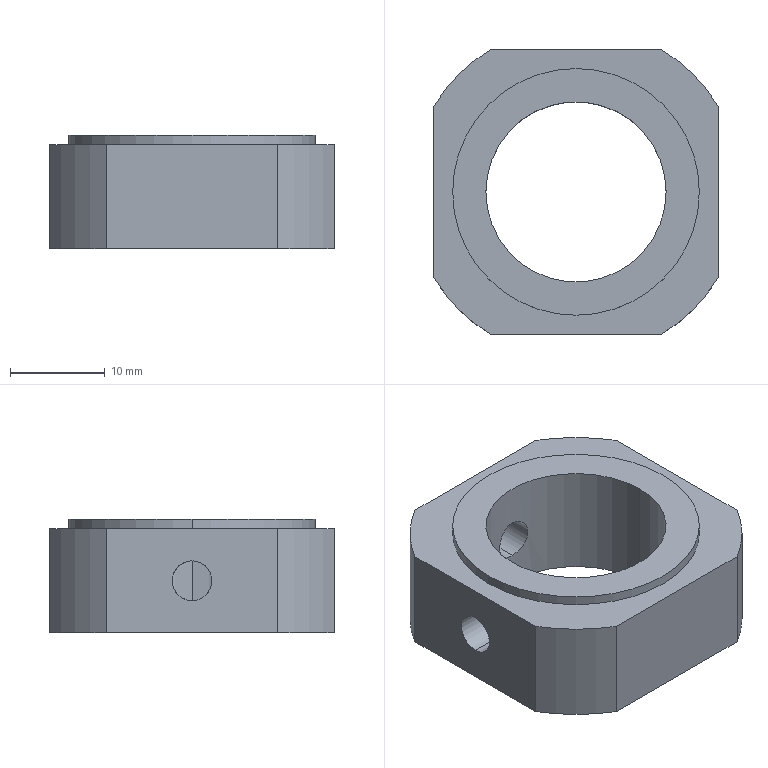Part | SolidWorks | features HoleWzd 2, ICE 2, Extrusion 1 | 1 solid | 19 faces | box 30 x 30 x 12 mm | volume 6216 mm3 | cylinder 12 | plane 7 | commonest cylinder face diameters 4.2 x4 35 x4 19 x2 26 x2
STEP:
#1=CARTESIAN_POINT('',(0.,9.5,3.4));
#2=VERTEX_POINT('',#1);
#3=CARTESIAN_POINT('',(0.,9.5,7.6));
#4=VERTEX_POINT('',#3);
#5=CARTESIAN_POINT('',(0.,9.5,3.4));
#6=CARTESIAN_POINT('',(-0.2745,9.5,3.4));
#7=CARTESIAN_POINT('',(-0.5516,9.487,3.455));
#8=CARTESIAN_POINT('',(-0.9309,9.455,3.613));
#9=CARTESIAN_POINT('',(-1.054,9.442,3.678));
#10=CARTESIAN_POINT('',(-1.282,9.414,3.831));
#11=CARTESIAN_POINT('',(-1.387,9.399,3.918));
#12=CARTESIAN_POINT('',(-1.581,9.368,4.111));
#13=CARTESIAN_POINT('',(-1.669,9.352,4.219));
#14=CARTESIAN_POINT('',(-1.821,9.324,4.446));
#15=CARTESIAN_POINT('',(-1.886,9.311,4.566));
#16=CARTESIAN_POINT('',(-2.045,9.278,4.949));
#17=CARTESIAN_POINT('',(-2.1,9.265,5.222));
#18=CARTESIAN_POINT('',(-2.1,9.265,5.638));
#19=CARTESIAN_POINT('',(-2.087,9.268,5.774));
#20=CARTESIAN_POINT('',(-2.033,9.28,6.044));
#21=CARTESIAN_POINT('',(-1.992,9.289,6.178));
#22=CARTESIAN_POINT('',(-1.887,9.311,6.431));
#23=CARTESIAN_POINT('',(-1.823,9.324,6.552));
#24=CARTESIAN_POINT('',(-1.67,9.352,6.78));
#25=CARTESIAN_POINT('',(-1.582,9.368,6.888));
#26=CARTESIAN_POINT('',(-1.293,9.414,7.177));
#27=CARTESIAN_POINT('',(-1.06,9.444,7.334));
#28=CARTESIAN_POINT('',(-0.6808,9.476,7.491));
#29=CARTESIAN_POINT('',(-0.5473,9.485,7.532));
#30=CARTESIAN_POINT('',(-0.2765,9.497,7.586));
#31=CARTESIAN_POINT('',(-0.1392,9.5,7.6));
#32=CARTESIAN_POINT('',(0.,9.5,7.6));
#33=B_SPLINE_CURVE_WITH_KNOTS('',3,(#5,#6,#7,#8,#9,#10,#11,#12,#13,#14,#15,#16,#17,#18,#19,#20,#21,#22,#23,#24,#25,#26,#27,#28,#29,#30,#31,#32),.UNSPECIFIED.,.F.,.F.,(4,2,2,2,2,2,2,2,2,2,2,2,2,4),(0.006586,0.007409,0.00782,0.008232,0.008644,0.009055,0.009878,0.01029,0.0107,0.01111,0.01152,0.01235,0.01276,0.01317),.UNSPECIFIED.);
#34=EDGE_CURVE('',#2,#4,#33,.T.);
#35=ORIENTED_EDGE('',*,*,#34,.F.);
#36=CARTESIAN_POINT('',(0.,15.,3.4));
#37=VERTEX_POINT('',#36);
#38=CARTESIAN_POINT('',(0.,15.,3.4));
#39=DIRECTION('',(0.,1.,0.));
#40=VECTOR('',#39,1000.);
#41=LINE('',#38,#40);
#42=EDGE_CURVE('',#2,#37,#41,.T.);
#43=ORIENTED_EDGE('',*,*,#42,.T.);
#44=CARTESIAN_POINT('',(0.,15.,7.6));
#45=VERTEX_POINT('',#44);
#46=CARTESIAN_POINT('',(0.,15.,5.5));
#47=DIRECTION('',(0.,1.,0.));
#48=DIRECTION('',(0.,0.,1.));
#49=AXIS2_PLACEMENT_3D('',#46,#47,#48);
#50=CIRCLE('',#49,2.1);
#51=EDGE_CURVE('',#37,#45,#50,.T.);
#52=ORIENTED_EDGE('',*,*,#51,.T.);
#53=CARTESIAN_POINT('',(0.,15.,7.6));
#54=DIRECTION('',(0.,1.,0.));
#55=VECTOR('',#54,1000.);
#56=LINE('',#53,#55);
#57=EDGE_CURVE('',#4,#45,#56,.T.);
#58=ORIENTED_EDGE('',*,*,#57,.F.);
#59=EDGE_LOOP('',(#35,#43,#52,#58));
#60=FACE_OUTER_BOUND('',#59,.T.);
#61=CARTESIAN_POINT('',(0.,15.,5.5));
#62=DIRECTION('',(0.,1.,0.));
#63=DIRECTION('',(0.,0.,1.));
#64=AXIS2_PLACEMENT_3D('',#61,#62,#63);
#65=CYLINDRICAL_SURFACE('',#64,2.1);
#66=ADVANCED_FACE('',(#60),#65,.F.);
#67=CARTESIAN_POINT('',(-9.5,0.,3.4));
#68=VERTEX_POINT('',#67);
#69=CARTESIAN_POINT('',(-9.5,0.,7.6));
#70=VERTEX_POINT('',#69);
#71=CARTESIAN_POINT('',(-9.5,0.,3.4));
#72=CARTESIAN_POINT('',(-9.5,-0.2745,3.4));
#73=CARTESIAN_POINT('',(-9.487,-0.5516,3.455));
#74=CARTESIAN_POINT('',(-9.455,-0.9309,3.613));
#75=CARTESIAN_POINT('',(-9.442,-1.054,3.678));
#76=CARTESIAN_POINT('',(-9.414,-1.282,3.831));
#77=CARTESIAN_POINT('',(-9.399,-1.387,3.918));
#78=CARTESIAN_POINT('',(-9.368,-1.581,4.111));
#79=CARTESIAN_POINT('',(-9.352,-1.669,4.219));
#80=CARTESIAN_POINT('',(-9.324,-1.821,4.446));
#81=CARTESIAN_POINT('',(-9.311,-1.886,4.566));
#82=CARTESIAN_POINT('',(-9.278,-2.045,4.949));
#83=CARTESIAN_POINT('',(-9.265,-2.1,5.222));
#84=CARTESIAN_POINT('',(-9.265,-2.1,5.638));
#85=CARTESIAN_POINT('',(-9.268,-2.087,5.774));
#86=CARTESIAN_POINT('',(-9.28,-2.033,6.044));
#87=CARTESIAN_POINT('',(-9.289,-1.992,6.178));
#88=CARTESIAN_POINT('',(-9.311,-1.887,6.431));
#89=CARTESIAN_POINT('',(-9.324,-1.823,6.552));
#90=CARTESIAN_POINT('',(-9.352,-1.67,6.78));
#91=CARTESIAN_POINT('',(-9.368,-1.582,6.888));
#92=CARTESIAN_POINT('',(-9.414,-1.293,7.177));
#93=CARTESIAN_POINT('',(-9.444,-1.06,7.334));
#94=CARTESIAN_POINT('',(-9.476,-0.6808,7.491));
#95=CARTESIAN_POINT('',(-9.485,-0.5473,7.532));
#96=CARTESIAN_POINT('',(-9.497,-0.2765,7.586));
#97=CARTESIAN_POINT('',(-9.5,-0.1392,7.6));
#98=CARTESIAN_POINT('',(-9.5,0.,7.6));
#99=B_SPLINE_CURVE_WITH_KNOTS('',3,(#71,#72,#73,#74,#75,#76,#77,#78,#79,#80,#81,#82,#83,#84,#85,#86,#87,#88,#89,#90,#91,#92,#93,#94,#95,#96,#97,#98),.UNSPECIFIED.,.F.,.F.,(4,2,2,2,2,2,2,2,2,2,2,2,2,4),(0.006586,0.007409,0.00782,0.008232,0.008644,0.009055,0.009878,0.01029,0.0107,0.01111,0.01152,0.01235,0.01276,0.01317),.UNSPECIFIED.);
#100=EDGE_CURVE('',#68,#70,#99,.T.);
#101=ORIENTED_EDGE('',*,*,#100,.F.);
#102=CARTESIAN_POINT('',(-15.,0.,3.4));
#103=VERTEX_POINT('',#102);
#104=CARTESIAN_POINT('',(-15.,0.,3.4));
#105=DIRECTION('',(-1.,0.,0.));
#106=VECTOR('',#105,1000.);
#107=LINE('',#104,#106);
#108=EDGE_CURVE('',#68,#103,#107,.T.);
#109=ORIENTED_EDGE('',*,*,#108,.T.);
#110=CARTESIAN_POINT('',(-15.,0.,7.6));
#111=VERTEX_POINT('',#110);
#112=CARTESIAN_POINT('',(-15.,0.,5.5));
#113=DIRECTION('',(-1.,0.,0.));
#114=DIRECTION('',(0.,0.,1.));
#115=AXIS2_PLACEMENT_3D('',#112,#113,#114);
#116=CIRCLE('',#115,2.1);
#117=EDGE_CURVE('',#103,#111,#116,.T.);
#118=ORIENTED_EDGE('',*,*,#117,.T.);
#119=CARTESIAN_POINT('',(-15.,0.,7.6));
#120=DIRECTION('',(-1.,0.,0.));
#121=VECTOR('',#120,1000.);
#122=LINE('',#119,#121);
#123=EDGE_CURVE('',#70,#111,#122,.T.);
#124=ORIENTED_EDGE('',*,*,#123,.F.);
#125=EDGE_LOOP('',(#101,#109,#118,#124));
#126=FACE_OUTER_BOUND('',#125,.T.);
#127=CARTESIAN_POINT('',(-15.,0.,5.5));
#128=DIRECTION('',(-1.,0.,0.));
#129=DIRECTION('',(0.,0.,1.));
#130=AXIS2_PLACEMENT_3D('',#127,#128,#129);
#131=CYLINDRICAL_SURFACE('',#130,2.1);
#132=ADVANCED_FACE('',(#126),#131,.F.);
#133=CARTESIAN_POINT('',(-9.5,0.,0.));
#134=VERTEX_POINT('',#133);
#135=CARTESIAN_POINT('',(9.5,0.,0.));
#136=VERTEX_POINT('',#135);
#137=CARTESIAN_POINT('',(0.,0.,0.));
#138=DIRECTION('',(0.,0.,1.));
#139=DIRECTION('',(1.,0.,0.));
#140=AXIS2_PLACEMENT_3D('',#137,#138,#139);
#141=CIRCLE('',#140,9.5);
#142=EDGE_CURVE('',#134,#136,#141,.T.);
#143=ORIENTED_EDGE('',*,*,#142,.F.);
#144=CARTESIAN_POINT('',(-9.5,0.,0.));
#145=DIRECTION('',(0.,0.,1.));
#146=VECTOR('',#145,1000.);
#147=LINE('',#144,#146);
#148=EDGE_CURVE('',#134,#68,#147,.T.);
#149=ORIENTED_EDGE('',*,*,#148,.T.);
#150=ORIENTED_EDGE('',*,*,#100,.T.);
#151=CARTESIAN_POINT('',(-9.5,0.,12.));
#152=VERTEX_POINT('',#151);
#153=CARTESIAN_POINT('',(-9.5,0.,0.));
#154=DIRECTION('',(0.,0.,1.));
#155=VECTOR('',#154,1000.);
#156=LINE('',#153,#155);
#157=EDGE_CURVE('',#70,#152,#156,.T.);
#158=ORIENTED_EDGE('',*,*,#157,.T.);
#159=CARTESIAN_POINT('',(9.5,0.,12.));
#160=VERTEX_POINT('',#159);
#161=CARTESIAN_POINT('',(0.,0.,12.));
#162=DIRECTION('',(0.,0.,1.));
#163=DIRECTION('',(1.,0.,0.));
#164=AXIS2_PLACEMENT_3D('',#161,#162,#163);
#165=CIRCLE('',#164,9.5);
#166=EDGE_CURVE('',#152,#160,#165,.T.);
#167=ORIENTED_EDGE('',*,*,#166,.T.);
#168=CARTESIAN_POINT('',(9.5,0.,0.));
#169=DIRECTION('',(0.,0.,1.));
#170=VECTOR('',#169,1000.);
#171=LINE('',#168,#170);
#172=EDGE_CURVE('',#136,#160,#171,.T.);
#173=ORIENTED_EDGE('',*,*,#172,.F.);
#174=EDGE_LOOP('',(#143,#149,#150,#158,#167,#173));
#175=FACE_OUTER_BOUND('',#174,.T.);
#176=CARTESIAN_POINT('',(0.,0.,0.));
#177=DIRECTION('',(0.,0.,1.));
#178=DIRECTION('',(1.,0.,0.));
#179=AXIS2_PLACEMENT_3D('',#176,#177,#178);
#180=CYLINDRICAL_SURFACE('',#179,9.5);
#181=ADVANCED_FACE('',(#175),#180,.F.);
#182=CARTESIAN_POINT('',(13.,0.,12.));
#183=VERTEX_POINT('',#182);
#184=CARTESIAN_POINT('',(-13.,0.,12.));
#185=VERTEX_POINT('',#184);
#186=CARTESIAN_POINT('',(0.,0.,12.));
#187=DIRECTION('',(0.,0.,1.));
#188=DIRECTION('',(1.,0.,0.));
#189=AXIS2_PLACEMENT_3D('',#186,#187,#188);
#190=CIRCLE('',#189,13.);
#191=EDGE_CURVE('',#183,#185,#190,.T.);
#192=ORIENTED_EDGE('',*,*,#191,.F.);
#193=CARTESIAN_POINT('',(13.,0.,11.));
#194=VERTEX_POINT('',#193);
#195=CARTESIAN_POINT('',(13.,0.,12.));
#196=DIRECTION('',(0.,0.,-1.));
#197=VECTOR('',#196,1000.);
#198=LINE('',#195,#197);
#199=EDGE_CURVE('',#183,#194,#198,.T.);
#200=ORIENTED_EDGE('',*,*,#199,.T.);
#201=CARTESIAN_POINT('',(-13.,0.,11.));
#202=VERTEX_POINT('',#201);
#203=CARTESIAN_POINT('',(0.,0.,11.));
#204=DIRECTION('',(0.,0.,1.));
#205=DIRECTION('',(1.,0.,0.));
#206=AXIS2_PLACEMENT_3D('',#203,#204,#205);
#207=CIRCLE('',#206,13.);
#208=EDGE_CURVE('',#194,#202,#207,.T.);
#209=ORIENTED_EDGE('',*,*,#208,.T.);
#210=CARTESIAN_POINT('',(-13.,0.,12.));
#211=DIRECTION('',(0.,0.,-1.));
#212=VECTOR('',#211,1000.);
#213=LINE('',#210,#212);
#214=EDGE_CURVE('',#185,#202,#213,.T.);
#215=ORIENTED_EDGE('',*,*,#214,.F.);
#216=EDGE_LOOP('',(#192,#200,#209,#215));
#217=FACE_OUTER_BOUND('',#216,.T.);
#218=CARTESIAN_POINT('',(0.,0.,12.));
#219=DIRECTION('',(0.,0.,-1.));
#220=DIRECTION('',(-1.,0.,0.));
#221=AXIS2_PLACEMENT_3D('',#218,#219,#220);
#222=CYLINDRICAL_SURFACE('',#221,13.);
#223=ADVANCED_FACE('',(#217),#222,.T.);
#224=CARTESIAN_POINT('',(-9.014,15.,11.));
#225=VERTEX_POINT('',#224);
#226=CARTESIAN_POINT('',(-15.,9.014,11.));
#227=VERTEX_POINT('',#226);
#228=CARTESIAN_POINT('',(0.,0.,11.));
#229=DIRECTION('',(0.,0.,1.));
#230=DIRECTION('',(1.,0.,0.));
#231=AXIS2_PLACEMENT_3D('',#228,#229,#230);
#232=CIRCLE('',#231,17.5);
#233=EDGE_CURVE('',#225,#227,#232,.T.);
#234=ORIENTED_EDGE('',*,*,#233,.T.);
#235=CARTESIAN_POINT('',(-15.,-9.014,11.));
#236=VERTEX_POINT('',#235);
#237=CARTESIAN_POINT('',(-15.,-9.014,11.));
#238=DIRECTION('',(0.,-1.,0.));
#239=VECTOR('',#238,1000.);
#240=LINE('',#237,#239);
#241=EDGE_CURVE('',#227,#236,#240,.T.);
#242=ORIENTED_EDGE('',*,*,#241,.T.);
#243=CARTESIAN_POINT('',(-9.014,-15.,11.));
#244=VERTEX_POINT('',#243);
#245=CARTESIAN_POINT('',(0.,0.,11.));
#246=DIRECTION('',(0.,0.,1.));
#247=DIRECTION('',(1.,0.,0.));
#248=AXIS2_PLACEMENT_3D('',#245,#246,#247);
#249=CIRCLE('',#248,17.5);
#250=EDGE_CURVE('',#236,#244,#249,.T.);
#251=ORIENTED_EDGE('',*,*,#250,.T.);
#252=CARTESIAN_POINT('',(9.014,-15.,11.));
#253=VERTEX_POINT('',#252);
#254=CARTESIAN_POINT('',(9.014,-15.,11.));
#255=DIRECTION('',(1.,0.,0.));
#256=VECTOR('',#255,1000.);
#257=LINE('',#254,#256);
#258=EDGE_CURVE('',#244,#253,#257,.T.);
#259=ORIENTED_EDGE('',*,*,#258,.T.);
#260=CARTESIAN_POINT('',(15.,-9.014,11.));
#261=VERTEX_POINT('',#260);
#262=CARTESIAN_POINT('',(0.,0.,11.));
#263=DIRECTION('',(0.,0.,1.));
#264=DIRECTION('',(1.,0.,0.));
#265=AXIS2_PLACEMENT_3D('',#262,#263,#264);
#266=CIRCLE('',#265,17.5);
#267=EDGE_CURVE('',#253,#261,#266,.T.);
#268=ORIENTED_EDGE('',*,*,#267,.T.);
#269=CARTESIAN_POINT('',(15.,9.014,11.));
#270=VERTEX_POINT('',#269);
#271=CARTESIAN_POINT('',(15.,9.014,11.));
#272=DIRECTION('',(0.,1.,0.));
#273=VECTOR('',#272,1000.);
#274=LINE('',#271,#273);
#275=EDGE_CURVE('',#261,#270,#274,.T.);
#276=ORIENTED_EDGE('',*,*,#275,.T.);
#277=CARTESIAN_POINT('',(9.014,15.,11.));
#278=VERTEX_POINT('',#277);
#279=CARTESIAN_POINT('',(0.,0.,11.));
#280=DIRECTION('',(0.,0.,1.));
#281=DIRECTION('',(1.,0.,0.));
#282=AXIS2_PLACEMENT_3D('',#279,#280,#281);
#283=CIRCLE('',#282,17.5);
#284=EDGE_CURVE('',#270,#278,#283,.T.);
#285=ORIENTED_EDGE('',*,*,#284,.T.);
#286=CARTESIAN_POINT('',(-9.014,15.,11.));
#287=DIRECTION('',(-1.,0.,0.));
#288=VECTOR('',#287,1000.);
#289=LINE('',#286,#288);
#290=EDGE_CURVE('',#278,#225,#289,.T.);
#291=ORIENTED_EDGE('',*,*,#290,.T.);
#292=EDGE_LOOP('',(#234,#242,#251,#259,#268,#276,#285,#291));
#293=FACE_OUTER_BOUND('',#292,.T.);
#294=CARTESIAN_POINT('',(0.,0.,11.));
#295=DIRECTION('',(0.,0.,1.));
#296=DIRECTION('',(1.,0.,0.));
#297=AXIS2_PLACEMENT_3D('',#294,#295,#296);
#298=CIRCLE('',#297,13.);
#299=EDGE_CURVE('',#202,#194,#298,.T.);
#300=ORIENTED_EDGE('',*,*,#299,.F.);
#301=ORIENTED_EDGE('',*,*,#208,.F.);
#302=EDGE_LOOP('',(#300,#301));
#303=FACE_BOUND('',#302,.T.);
#304=CARTESIAN_POINT('',(0.,0.,11.));
#305=DIRECTION('',(0.,0.,1.));
#306=DIRECTION('',(1.,0.,0.));
#307=AXIS2_PLACEMENT_3D('',#304,#305,#306);
#308=PLANE('',#307);
#309=ADVANCED_FACE('',(#293,#303),#308,.T.);
#310=CARTESIAN_POINT('',(-9.014,15.,0.));
#311=VERTEX_POINT('',#310);
#312=CARTESIAN_POINT('',(-15.,9.014,0.));
#313=VERTEX_POINT('',#312);
#314=CARTESIAN_POINT('',(0.,0.,0.));
#315=DIRECTION('',(0.,0.,1.));
#316=DIRECTION('',(1.,0.,0.));
#317=AXIS2_PLACEMENT_3D('',#314,#315,#316);
#318=CIRCLE('',#317,17.5);
#319=EDGE_CURVE('',#311,#313,#318,.T.);
#320=ORIENTED_EDGE('',*,*,#319,.T.);
#321=CARTESIAN_POINT('',(-15.,9.014,11.));
#322=DIRECTION('',(0.,0.,-1.));
#323=VECTOR('',#322,1000.);
#324=LINE('',#321,#323);
#325=EDGE_CURVE('',#227,#313,#324,.T.);
#326=ORIENTED_EDGE('',*,*,#325,.F.);
#327=ORIENTED_EDGE('',*,*,#233,.F.);
#328=CARTESIAN_POINT('',(-9.014,15.,11.));
#329=DIRECTION('',(0.,0.,-1.));
#330=VECTOR('',#329,1000.);
#331=LINE('',#328,#330);
#332=EDGE_CURVE('',#225,#311,#331,.T.);
#333=ORIENTED_EDGE('',*,*,#332,.T.);
#334=EDGE_LOOP('',(#320,#326,#327,#333));
#335=FACE_OUTER_BOUND('',#334,.T.);
#336=CARTESIAN_POINT('',(0.,0.,11.));
#337=DIRECTION('',(0.,0.,-1.));
#338=DIRECTION('',(-1.,0.,0.));
#339=AXIS2_PLACEMENT_3D('',#336,#337,#338);
#340=CYLINDRICAL_SURFACE('',#339,17.5);
#341=ADVANCED_FACE('',(#335),#340,.T.);
#342=CARTESIAN_POINT('',(-15.,0.,5.5));
#343=DIRECTION('',(-1.,0.,0.));
#344=DIRECTION('',(0.,0.,1.));
#345=AXIS2_PLACEMENT_3D('',#342,#343,#344);
#346=CIRCLE('',#345,2.1);
#347=EDGE_CURVE('',#111,#103,#346,.T.);
#348=ORIENTED_EDGE('',*,*,#347,.F.);
#349=ORIENTED_EDGE('',*,*,#117,.F.);
#350=EDGE_LOOP('',(#348,#349));
#351=FACE_BOUND('',#350,.T.);
#352=CARTESIAN_POINT('',(-15.,-9.014,0.));
#353=VERTEX_POINT('',#352);
#354=CARTESIAN_POINT('',(-15.,-9.014,0.));
#355=DIRECTION('',(0.,-1.,0.));
#356=VECTOR('',#355,1000.);
#357=LINE('',#354,#356);
#358=EDGE_CURVE('',#313,#353,#357,.T.);
#359=ORIENTED_EDGE('',*,*,#358,.T.);
#360=CARTESIAN_POINT('',(-15.,-9.014,11.));
#361=DIRECTION('',(0.,0.,-1.));
#362=VECTOR('',#361,1000.);
#363=LINE('',#360,#362);
#364=EDGE_CURVE('',#236,#353,#363,.T.);
#365=ORIENTED_EDGE('',*,*,#364,.F.);
#366=ORIENTED_EDGE('',*,*,#241,.F.);
#367=ORIENTED_EDGE('',*,*,#325,.T.);
#368=EDGE_LOOP('',(#359,#365,#366,#367));
#369=FACE_OUTER_BOUND('',#368,.T.);
#370=CARTESIAN_POINT('',(-15.,-9.014,11.));
#371=DIRECTION('',(1.,0.,0.));
#372=DIRECTION('',(0.,1.,0.));
#373=AXIS2_PLACEMENT_3D('',#370,#371,#372);
#374=PLANE('',#373);
#375=ADVANCED_FACE('',(#351,#369),#374,.F.);
#376=CARTESIAN_POINT('',(-9.014,-15.,0.));
#377=VERTEX_POINT('',#376);
#378=CARTESIAN_POINT('',(0.,0.,0.));
#379=DIRECTION('',(0.,0.,1.));
#380=DIRECTION('',(1.,0.,0.));
#381=AXIS2_PLACEMENT_3D('',#378,#379,#380);
#382=CIRCLE('',#381,17.5);
#383=EDGE_CURVE('',#353,#377,#382,.T.);
#384=ORIENTED_EDGE('',*,*,#383,.T.);
#385=CARTESIAN_POINT('',(-9.014,-15.,11.));
#386=DIRECTION('',(0.,0.,-1.));
#387=VECTOR('',#386,1000.);
#388=LINE('',#385,#387);
#389=EDGE_CURVE('',#244,#377,#388,.T.);
#390=ORIENTED_EDGE('',*,*,#389,.F.);
#391=ORIENTED_EDGE('',*,*,#250,.F.);
#392=ORIENTED_EDGE('',*,*,#364,.T.);
#393=EDGE_LOOP('',(#384,#390,#391,#392));
#394=FACE_OUTER_BOUND('',#393,.T.);
#395=CARTESIAN_POINT('',(0.,0.,11.));
#396=DIRECTION('',(0.,0.,-1.));
#397=DIRECTION('',(-1.,0.,0.));
#398=AXIS2_PLACEMENT_3D('',#395,#396,#397);
#399=CYLINDRICAL_SURFACE('',#398,17.5);
#400=ADVANCED_FACE('',(#394),#399,.T.);
#401=CARTESIAN_POINT('',(9.014,-15.,0.));
#402=VERTEX_POINT('',#401);
#403=CARTESIAN_POINT('',(9.014,-15.,0.));
#404=DIRECTION('',(1.,0.,0.));
#405=VECTOR('',#404,1000.);
#406=LINE('',#403,#405);
#407=EDGE_CURVE('',#377,#402,#406,.T.);
#408=ORIENTED_EDGE('',*,*,#407,.T.);
#409=CARTESIAN_POINT('',(9.014,-15.,11.));
#410=DIRECTION('',(0.,0.,-1.));
#411=VECTOR('',#410,1000.);
#412=LINE('',#409,#411);
#413=EDGE_CURVE('',#253,#402,#412,.T.);
#414=ORIENTED_EDGE('',*,*,#413,.F.);
#415=ORIENTED_EDGE('',*,*,#258,.F.);
#416=ORIENTED_EDGE('',*,*,#389,.T.);
#417=EDGE_LOOP('',(#408,#414,#415,#416));
#418=FACE_OUTER_BOUND('',#417,.T.);
#419=CARTESIAN_POINT('',(9.014,-15.,11.));
#420=DIRECTION('',(0.,1.,0.));
#421=DIRECTION('',(0.,0.,1.));
#422=AXIS2_PLACEMENT_3D('',#419,#420,#421);
#423=PLANE('',#422);
#424=ADVANCED_FACE('',(#418),#423,.F.);
#425=CARTESIAN_POINT('',(15.,-9.014,0.));
#426=VERTEX_POINT('',#425);
#427=CARTESIAN_POINT('',(0.,0.,0.));
#428=DIRECTION('',(0.,0.,1.));
#429=DIRECTION('',(1.,0.,0.));
#430=AXIS2_PLACEMENT_3D('',#427,#428,#429);
#431=CIRCLE('',#430,17.5);
#432=EDGE_CURVE('',#402,#426,#431,.T.);
#433=ORIENTED_EDGE('',*,*,#432,.T.);
#434=CARTESIAN_POINT('',(15.,-9.014,11.));
#435=DIRECTION('',(0.,0.,-1.));
#436=VECTOR('',#435,1000.);
#437=LINE('',#434,#436);
#438=EDGE_CURVE('',#261,#426,#437,.T.);
#439=ORIENTED_EDGE('',*,*,#438,.F.);
#440=ORIENTED_EDGE('',*,*,#267,.F.);
#441=ORIENTED_EDGE('',*,*,#413,.T.);
#442=EDGE_LOOP('',(#433,#439,#440,#441));
#443=FACE_OUTER_BOUND('',#442,.T.);
#444=CARTESIAN_POINT('',(0.,0.,11.));
#445=DIRECTION('',(0.,0.,-1.));
#446=DIRECTION('',(-1.,0.,0.));
#447=AXIS2_PLACEMENT_3D('',#444,#445,#446);
#448=CYLINDRICAL_SURFACE('',#447,17.5);
#449=ADVANCED_FACE('',(#443),#448,.T.);
#450=CARTESIAN_POINT('',(15.,9.014,0.));
#451=VERTEX_POINT('',#450);
#452=CARTESIAN_POINT('',(15.,9.014,0.));
#453=DIRECTION('',(0.,1.,0.));
#454=VECTOR('',#453,1000.);
#455=LINE('',#452,#454);
#456=EDGE_CURVE('',#426,#451,#455,.T.);
#457=ORIENTED_EDGE('',*,*,#456,.T.);
#458=CARTESIAN_POINT('',(15.,9.014,11.));
#459=DIRECTION('',(0.,0.,-1.));
#460=VECTOR('',#459,1000.);
#461=LINE('',#458,#460);
#462=EDGE_CURVE('',#270,#451,#461,.T.);
#463=ORIENTED_EDGE('',*,*,#462,.F.);
#464=ORIENTED_EDGE('',*,*,#275,.F.);
#465=ORIENTED_EDGE('',*,*,#438,.T.);
#466=EDGE_LOOP('',(#457,#463,#464,#465));
#467=FACE_OUTER_BOUND('',#466,.T.);
#468=CARTESIAN_POINT('',(15.,9.014,11.));
#469=DIRECTION('',(-1.,0.,0.));
#470=DIRECTION('',(0.,-1.,0.));
#471=AXIS2_PLACEMENT_3D('',#468,#469,#470);
#472=PLANE('',#471);
#473=ADVANCED_FACE('',(#467),#472,.F.);
#474=CARTESIAN_POINT('',(9.014,15.,0.));
#475=VERTEX_POINT('',#474);
#476=CARTESIAN_POINT('',(0.,0.,0.));
#477=DIRECTION('',(0.,0.,1.));
#478=DIRECTION('',(1.,0.,0.));
#479=AXIS2_PLACEMENT_3D('',#476,#477,#478);
#480=CIRCLE('',#479,17.5);
#481=EDGE_CURVE('',#451,#475,#480,.T.);
#482=ORIENTED_EDGE('',*,*,#481,.T.);
#483=CARTESIAN_POINT('',(9.014,15.,11.));
#484=DIRECTION('',(0.,0.,-1.));
#485=VECTOR('',#484,1000.);
#486=LINE('',#483,#485);
#487=EDGE_CURVE('',#278,#475,#486,.T.);
#488=ORIENTED_EDGE('',*,*,#487,.F.);
#489=ORIENTED_EDGE('',*,*,#284,.F.);
#490=ORIENTED_EDGE('',*,*,#462,.T.);
#491=EDGE_LOOP('',(#482,#488,#489,#490));
#492=FACE_OUTER_BOUND('',#491,.T.);
#493=CARTESIAN_POINT('',(0.,0.,11.));
#494=DIRECTION('',(0.,0.,-1.));
#495=DIRECTION('',(-1.,0.,0.));
#496=AXIS2_PLACEMENT_3D('',#493,#494,#495);
#497=CYLINDRICAL_SURFACE('',#496,17.5);
#498=ADVANCED_FACE('',(#492),#497,.T.);
#499=CARTESIAN_POINT('',(0.,15.,5.5));
#500=DIRECTION('',(0.,1.,0.));
#501=DIRECTION('',(0.,0.,1.));
#502=AXIS2_PLACEMENT_3D('',#499,#500,#501);
#503=CIRCLE('',#502,2.1);
#504=EDGE_CURVE('',#45,#37,#503,.T.);
#505=ORIENTED_EDGE('',*,*,#504,.F.);
#506=ORIENTED_EDGE('',*,*,#51,.F.);
#507=EDGE_LOOP('',(#505,#506));
#508=FACE_BOUND('',#507,.T.);
#509=CARTESIAN_POINT('',(-9.014,15.,0.));
#510=DIRECTION('',(-1.,0.,0.));
#511=VECTOR('',#510,1000.);
#512=LINE('',#509,#511);
#513=EDGE_CURVE('',#475,#311,#512,.T.);
#514=ORIENTED_EDGE('',*,*,#513,.T.);
#515=ORIENTED_EDGE('',*,*,#332,.F.);
#516=ORIENTED_EDGE('',*,*,#290,.F.);
#517=ORIENTED_EDGE('',*,*,#487,.T.);
#518=EDGE_LOOP('',(#514,#515,#516,#517));
#519=FACE_OUTER_BOUND('',#518,.T.);
#520=CARTESIAN_POINT('',(-9.014,15.,11.));
#521=DIRECTION('',(0.,-1.,0.));
#522=DIRECTION('',(0.,0.,-1.));
#523=AXIS2_PLACEMENT_3D('',#520,#521,#522);
#524=PLANE('',#523);
#525=ADVANCED_FACE('',(#508,#519),#524,.F.);
#526=CARTESIAN_POINT('',(0.,0.,0.));
#527=DIRECTION('',(0.,0.,1.));
#528=DIRECTION('',(1.,0.,0.));
#529=AXIS2_PLACEMENT_3D('',#526,#527,#528);
#530=CIRCLE('',#529,9.5);
#531=EDGE_CURVE('',#136,#134,#530,.T.);
#532=ORIENTED_EDGE('',*,*,#531,.T.);
#533=ORIENTED_EDGE('',*,*,#142,.T.);
#534=EDGE_LOOP('',(#532,#533));
#535=FACE_BOUND('',#534,.T.);
#536=ORIENTED_EDGE('',*,*,#319,.F.);
#537=ORIENTED_EDGE('',*,*,#513,.F.);
#538=ORIENTED_EDGE('',*,*,#481,.F.);
#539=ORIENTED_EDGE('',*,*,#456,.F.);
#540=ORIENTED_EDGE('',*,*,#432,.F.);
#541=ORIENTED_EDGE('',*,*,#407,.F.);
#542=ORIENTED_EDGE('',*,*,#383,.F.);
#543=ORIENTED_EDGE('',*,*,#358,.F.);
#544=EDGE_LOOP('',(#536,#537,#538,#539,#540,#541,#542,#543));
#545=FACE_OUTER_BOUND('',#544,.T.);
#546=CARTESIAN_POINT('',(0.,0.,0.));
#547=DIRECTION('',(0.,0.,1.));
#548=DIRECTION('',(1.,0.,0.));
#549=AXIS2_PLACEMENT_3D('',#546,#547,#548);
#550=PLANE('',#549);
#551=ADVANCED_FACE('',(#535,#545),#550,.F.);
#552=ORIENTED_EDGE('',*,*,#199,.F.);
#553=CARTESIAN_POINT('',(0.,0.,12.));
#554=DIRECTION('',(0.,0.,1.));
#555=DIRECTION('',(1.,0.,0.));
#556=AXIS2_PLACEMENT_3D('',#553,#554,#555);
#557=CIRCLE('',#556,13.);
#558=EDGE_CURVE('',#185,#183,#557,.T.);
#559=ORIENTED_EDGE('',*,*,#558,.F.);
#560=ORIENTED_EDGE('',*,*,#214,.T.);
#561=ORIENTED_EDGE('',*,*,#299,.T.);
#562=EDGE_LOOP('',(#552,#559,#560,#561));
#563=FACE_OUTER_BOUND('',#562,.T.);
#564=CARTESIAN_POINT('',(0.,0.,12.));
#565=DIRECTION('',(0.,0.,-1.));
#566=DIRECTION('',(-1.,0.,0.));
#567=AXIS2_PLACEMENT_3D('',#564,#565,#566);
#568=CYLINDRICAL_SURFACE('',#567,13.);
#569=ADVANCED_FACE('',(#563),#568,.T.);
#570=CARTESIAN_POINT('',(0.,0.,12.));
#571=DIRECTION('',(0.,0.,1.));
#572=DIRECTION('',(1.,0.,0.));
#573=AXIS2_PLACEMENT_3D('',#570,#571,#572);
#574=CIRCLE('',#573,9.5);
#575=EDGE_CURVE('',#160,#152,#574,.T.);
#576=ORIENTED_EDGE('',*,*,#575,.F.);
#577=ORIENTED_EDGE('',*,*,#166,.F.);
#578=EDGE_LOOP('',(#576,#577));
#579=FACE_BOUND('',#578,.T.);
#580=ORIENTED_EDGE('',*,*,#558,.T.);
#581=ORIENTED_EDGE('',*,*,#191,.T.);
#582=EDGE_LOOP('',(#580,#581));
#583=FACE_OUTER_BOUND('',#582,.T.);
#584=CARTESIAN_POINT('',(0.,0.,12.));
#585=DIRECTION('',(0.,0.,1.));
#586=DIRECTION('',(1.,0.,0.));
#587=AXIS2_PLACEMENT_3D('',#584,#585,#586);
#588=PLANE('',#587);
#589=ADVANCED_FACE('',(#579,#583),#588,.T.);
#590=ORIENTED_EDGE('',*,*,#148,.F.);
#591=ORIENTED_EDGE('',*,*,#531,.F.);
#592=ORIENTED_EDGE('',*,*,#172,.T.);
#593=ORIENTED_EDGE('',*,*,#575,.T.);
#594=ORIENTED_EDGE('',*,*,#157,.F.);
#595=CARTESIAN_POINT('',(-9.5,0.,7.6));
#596=CARTESIAN_POINT('',(-9.5,0.1392,7.6));
#597=CARTESIAN_POINT('',(-9.497,0.276,7.586));
#598=CARTESIAN_POINT('',(-9.485,0.545,7.533));
#599=CARTESIAN_POINT('',(-9.477,0.6787,7.492));
#600=CARTESIAN_POINT('',(-9.455,0.9328,7.386));
#601=CARTESIAN_POINT('',(-9.442,1.053,7.322));
#602=CARTESIAN_POINT('',(-9.414,1.281,7.17));
#603=CARTESIAN_POINT('',(-9.398,1.389,7.081));
#604=CARTESIAN_POINT('',(-9.353,1.678,6.791));
#605=CARTESIAN_POINT('',(-9.322,1.835,6.558));
#606=CARTESIAN_POINT('',(-9.289,1.992,6.179));
#607=CARTESIAN_POINT('',(-9.28,2.032,6.046));
#608=CARTESIAN_POINT('',(-9.268,2.087,5.775));
#609=CARTESIAN_POINT('',(-9.265,2.1,5.638));
#610=CARTESIAN_POINT('',(-9.265,2.1,5.363));
#611=CARTESIAN_POINT('',(-9.268,2.086,5.224));
#612=CARTESIAN_POINT('',(-9.28,2.032,4.954));
#613=CARTESIAN_POINT('',(-9.289,1.993,4.823));
#614=CARTESIAN_POINT('',(-9.322,1.834,4.441));
#615=CARTESIAN_POINT('',(-9.352,1.68,4.21));
#616=CARTESIAN_POINT('',(-9.399,1.387,3.917));
#617=CARTESIAN_POINT('',(-9.414,1.282,3.831));
#618=CARTESIAN_POINT('',(-9.442,1.055,3.679));
#619=CARTESIAN_POINT('',(-9.455,0.9315,3.613));
#620=CARTESIAN_POINT('',(-9.477,0.6778,3.508));
#621=CARTESIAN_POINT('',(-9.485,0.5469,3.468));
#622=CARTESIAN_POINT('',(-9.497,0.2767,3.414));
#623=CARTESIAN_POINT('',(-9.5,0.1373,3.4));
#624=CARTESIAN_POINT('',(-9.5,0.,3.4));
#625=B_SPLINE_CURVE_WITH_KNOTS('',3,(#595,#596,#597,#598,#599,#600,#601,#602,#603,#604,#605,#606,#607,#608,#609,#610,#611,#612,#613,#614,#615,#616,#617,#618,#619,#620,#621,#622,#623,#624),.UNSPECIFIED.,.F.,.F.,(4,2,2,2,2,2,2,2,2,2,2,2,2,2,4),(0.,0.0004116,0.0008232,0.001235,0.001646,0.00247,0.002881,0.003293,0.003705,0.004116,0.004939,0.005351,0.005763,0.006174,0.006586),.UNSPECIFIED.);
#626=EDGE_CURVE('',#70,#68,#625,.T.);
#627=ORIENTED_EDGE('',*,*,#626,.T.);
#628=EDGE_LOOP('',(#590,#591,#592,#593,#594,#627));
#629=FACE_OUTER_BOUND('',#628,.T.);
#630=CARTESIAN_POINT('',(0.,9.5,7.6));
#631=CARTESIAN_POINT('',(0.1392,9.5,7.6));
#632=CARTESIAN_POINT('',(0.276,9.497,7.586));
#633=CARTESIAN_POINT('',(0.545,9.485,7.533));
#634=CARTESIAN_POINT('',(0.6787,9.477,7.492));
#635=CARTESIAN_POINT('',(0.9328,9.455,7.386));
#636=CARTESIAN_POINT('',(1.053,9.442,7.322));
#637=CARTESIAN_POINT('',(1.281,9.414,7.17));
#638=CARTESIAN_POINT('',(1.389,9.398,7.081));
#639=CARTESIAN_POINT('',(1.678,9.353,6.791));
#640=CARTESIAN_POINT('',(1.835,9.322,6.558));
#641=CARTESIAN_POINT('',(1.992,9.289,6.179));
#642=CARTESIAN_POINT('',(2.032,9.28,6.046));
#643=CARTESIAN_POINT('',(2.087,9.268,5.775));
#644=CARTESIAN_POINT('',(2.1,9.265,5.638));
#645=CARTESIAN_POINT('',(2.1,9.265,5.363));
#646=CARTESIAN_POINT('',(2.086,9.268,5.224));
#647=CARTESIAN_POINT('',(2.032,9.28,4.954));
#648=CARTESIAN_POINT('',(1.993,9.289,4.823));
#649=CARTESIAN_POINT('',(1.834,9.322,4.441));
#650=CARTESIAN_POINT('',(1.68,9.352,4.21));
#651=CARTESIAN_POINT('',(1.387,9.399,3.917));
#652=CARTESIAN_POINT('',(1.282,9.414,3.831));
#653=CARTESIAN_POINT('',(1.055,9.442,3.679));
#654=CARTESIAN_POINT('',(0.9315,9.455,3.613));
#655=CARTESIAN_POINT('',(0.6778,9.477,3.508));
#656=CARTESIAN_POINT('',(0.5469,9.485,3.468));
#657=CARTESIAN_POINT('',(0.2767,9.497,3.414));
#658=CARTESIAN_POINT('',(0.1373,9.5,3.4));
#659=CARTESIAN_POINT('',(0.,9.5,3.4));
#660=B_SPLINE_CURVE_WITH_KNOTS('',3,(#630,#631,#632,#633,#634,#635,#636,#637,#638,#639,#640,#641,#642,#643,#644,#645,#646,#647,#648,#649,#650,#651,#652,#653,#654,#655,#656,#657,#658,#659),.UNSPECIFIED.,.F.,.F.,(4,2,2,2,2,2,2,2,2,2,2,2,2,2,4),(0.,0.0004116,0.0008232,0.001235,0.001646,0.00247,0.002881,0.003293,0.003705,0.004116,0.004939,0.005351,0.005763,0.006174,0.006586),.UNSPECIFIED.);
#661=EDGE_CURVE('',#4,#2,#660,.T.);
#662=ORIENTED_EDGE('',*,*,#661,.T.);
#663=ORIENTED_EDGE('',*,*,#34,.T.);
#664=EDGE_LOOP('',(#662,#663));
#665=FACE_BOUND('',#664,.T.);
#666=CARTESIAN_POINT('',(0.,0.,0.));
#667=DIRECTION('',(0.,0.,1.));
#668=DIRECTION('',(1.,0.,0.));
#669=AXIS2_PLACEMENT_3D('',#666,#667,#668);
#670=CYLINDRICAL_SURFACE('',#669,9.5);
#671=ADVANCED_FACE('',(#629,#665),#670,.F.);
#672=ORIENTED_EDGE('',*,*,#108,.F.);
#673=ORIENTED_EDGE('',*,*,#626,.F.);
#674=ORIENTED_EDGE('',*,*,#123,.T.);
#675=ORIENTED_EDGE('',*,*,#347,.T.);
#676=EDGE_LOOP('',(#672,#673,#674,#675));
#677=FACE_OUTER_BOUND('',#676,.T.);
#678=CARTESIAN_POINT('',(-15.,0.,5.5));
#679=DIRECTION('',(-1.,0.,0.));
#680=DIRECTION('',(0.,0.,1.));
#681=AXIS2_PLACEMENT_3D('',#678,#679,#680);
#682=CYLINDRICAL_SURFACE('',#681,2.1);
#683=ADVANCED_FACE('',(#677),#682,.F.);
#684=ORIENTED_EDGE('',*,*,#42,.F.);
#685=ORIENTED_EDGE('',*,*,#661,.F.);
#686=ORIENTED_EDGE('',*,*,#57,.T.);
#687=ORIENTED_EDGE('',*,*,#504,.T.);
#688=EDGE_LOOP('',(#684,#685,#686,#687));
#689=FACE_OUTER_BOUND('',#688,.T.);
#690=CARTESIAN_POINT('',(0.,15.,5.5));
#691=DIRECTION('',(0.,1.,0.));
#692=DIRECTION('',(0.,0.,1.));
#693=AXIS2_PLACEMENT_3D('',#690,#691,#692);
#694=CYLINDRICAL_SURFACE('',#693,2.1);
#695=ADVANCED_FACE('',(#689),#694,.F.);
#696=CLOSED_SHELL('',(#66,#132,#181,#223,#309,#341,#375,#400,#424,#449,#473,#498,#525,#551,#569,#589,#671,#683,#695));
#697=MANIFOLD_SOLID_BREP('',#696);
#698=CARTESIAN_POINT('',(0.,0.,0.));
#699=DIRECTION('',(0.,0.,1.));
#700=DIRECTION('',(1.,0.,0.));
#701=AXIS2_PLACEMENT_3D('',#698,#699,#700);
#702=(LENGTH_UNIT()NAMED_UNIT(*)SI_UNIT(.MILLI.,.METRE.));
#703=UNCERTAINTY_MEASURE_WITH_UNIT(LENGTH_MEASURE(0.00001),#702,'','');
#704=(NAMED_UNIT(*)PLANE_ANGLE_UNIT()SI_UNIT($,.RADIAN.));
#705=(NAMED_UNIT(*)SI_UNIT($,.STERADIAN.)SOLID_ANGLE_UNIT());
#706=(GEOMETRIC_REPRESENTATION_CONTEXT(3)GLOBAL_UNCERTAINTY_ASSIGNED_CONTEXT((#703))GLOBAL_UNIT_ASSIGNED_CONTEXT((#702,#704,#705))REPRESENTATION_CONTEXT('',''));
#707=ADVANCED_BREP_SHAPE_REPRESENTATION('',(#697,#701),#706);